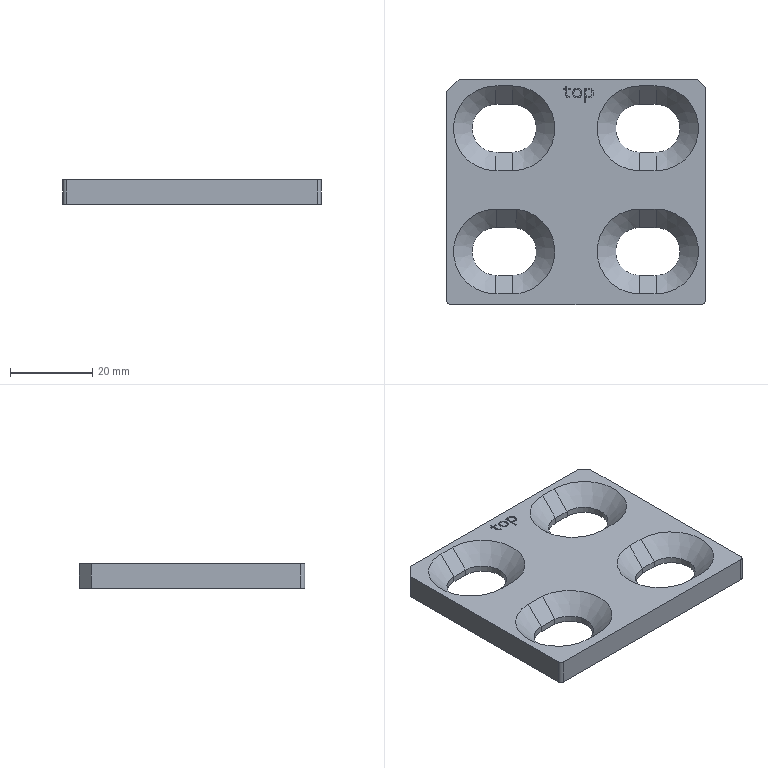Part | NX | features solid 2 | 1 solid | 154 faces | box 63 x 55 x 6 mm | volume 14849 mm3 | plane 136 | cylinder 10 | cone 8 | commonest cylinder face diameters 11.7 x8 2 x2